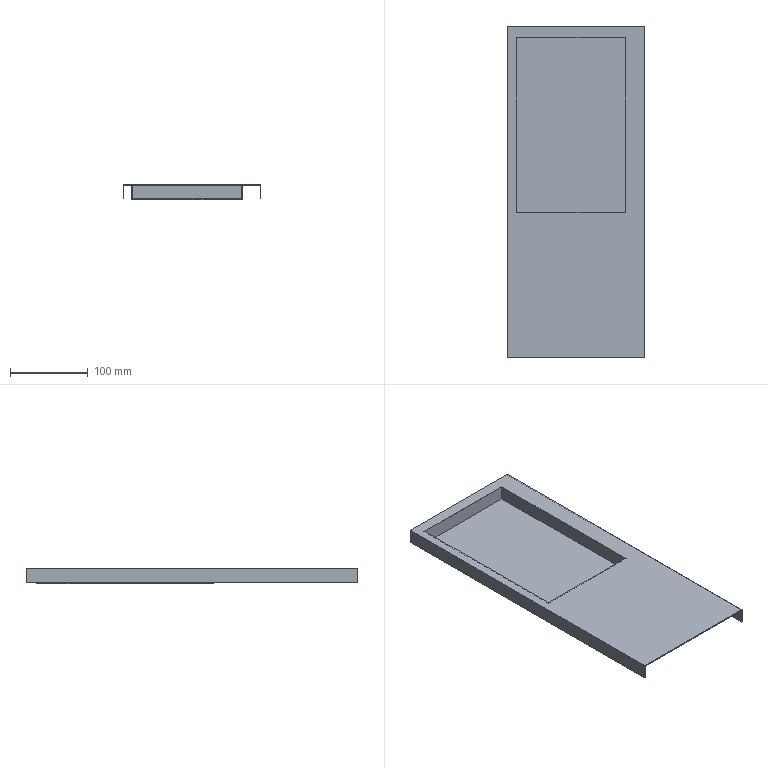Part | STEP file | Chassis front plate_RR | 1 solid | 20 faces | box 177 x 427 x 20 mm | volume 104897 mm3 | plane 20
STEP:
#1=CARTESIAN_POINT('',(0.,0.,0.));
#2=DIRECTION('',(0.,0.,1.));
#3=DIRECTION('',(1.,0.,0.));
#4=AXIS2_PLACEMENT_3D('',#1,#2,#3);
#5=CARTESIAN_POINT('',(-76.5,-26.5,0.));
#6=VERTEX_POINT('',#5);
#7=CARTESIAN_POINT('',(-76.5,198.5,0.));
#8=VERTEX_POINT('',#7);
#9=CARTESIAN_POINT('',(-76.5,-213.5,0.));
#10=DIRECTION('',(0.,1.,0.));
#11=VECTOR('',#10,1.);
#12=LINE('',#9,#11);
#13=CARTESIAN_POINT('',(-88.5,-213.5,0.));
#14=DIRECTION('',(0.,0.,1.));
#15=DIRECTION('',(1.,0.,0.));
#16=AXIS2_PLACEMENT_3D('',#13,#14,#15);
#17=PLANE('',#16);
#18=CARTESIAN_POINT('',(12.,0.));
#19=DIRECTION('',(0.,1.));
#20=VECTOR('',#19,1.);
#21=LINE('',#18,#20);
#22=(GEOMETRIC_REPRESENTATION_CONTEXT(2)PARAMETRIC_REPRESENTATION_CONTEXT()REPRESENTATION_CONTEXT('',''));
#23=DEFINITIONAL_REPRESENTATION('',(#21),#22);
#24=PCURVE('',#17,#23);
#25=CARTESIAN_POINT('',(-76.5,198.5,0.));
#26=DIRECTION('',(-1.,0.,0.));
#27=DIRECTION('',(0.,0.,1.));
#28=AXIS2_PLACEMENT_3D('',#25,#26,#27);
#29=PLANE('',#28);
#30=CARTESIAN_POINT('',(0.,-412.));
#31=DIRECTION('',(0.,1.));
#32=VECTOR('',#31,1.);
#33=LINE('',#30,#32);
#34=(GEOMETRIC_REPRESENTATION_CONTEXT(2)PARAMETRIC_REPRESENTATION_CONTEXT()REPRESENTATION_CONTEXT('',''));
#35=DEFINITIONAL_REPRESENTATION('',(#33),#34);
#36=PCURVE('',#29,#35);
#37=SURFACE_CURVE('',#12,(#24,#36),.PCURVE_S1.);
#38=EDGE_CURVE('',#6,#8,#37,.T.);
#39=ORIENTED_EDGE('',*,*,#38,.T.);
#40=CARTESIAN_POINT('',(63.5,198.5,0.));
#41=VERTEX_POINT('',#40);
#42=CARTESIAN_POINT('',(-88.5,198.5,0.));
#43=DIRECTION('',(1.,0.,0.));
#44=VECTOR('',#43,1.);
#45=LINE('',#42,#44);
#46=CARTESIAN_POINT('',(0.,412.));
#47=DIRECTION('',(1.,0.));
#48=VECTOR('',#47,1.);
#49=LINE('',#46,#48);
#50=(GEOMETRIC_REPRESENTATION_CONTEXT(2)PARAMETRIC_REPRESENTATION_CONTEXT()REPRESENTATION_CONTEXT('',''));
#51=DEFINITIONAL_REPRESENTATION('',(#49),#50);
#52=PCURVE('',#17,#51);
#53=CARTESIAN_POINT('',(63.5,198.5,0.));
#54=DIRECTION('',(0.,1.,0.));
#55=DIRECTION('',(0.,0.,1.));
#56=AXIS2_PLACEMENT_3D('',#53,#54,#55);
#57=PLANE('',#56);
#58=CARTESIAN_POINT('',(0.,-152.));
#59=DIRECTION('',(0.,1.));
#60=VECTOR('',#59,1.);
#61=LINE('',#58,#60);
#62=(GEOMETRIC_REPRESENTATION_CONTEXT(2)PARAMETRIC_REPRESENTATION_CONTEXT()REPRESENTATION_CONTEXT('',''));
#63=DEFINITIONAL_REPRESENTATION('',(#61),#62);
#64=PCURVE('',#57,#63);
#65=SURFACE_CURVE('',#45,(#52,#64),.PCURVE_S1.);
#66=EDGE_CURVE('',#8,#41,#65,.T.);
#67=ORIENTED_EDGE('',*,*,#66,.T.);
#68=CARTESIAN_POINT('',(63.5,-26.5,0.));
#69=VERTEX_POINT('',#68);
#70=CARTESIAN_POINT('',(63.5,-213.5,0.));
#71=DIRECTION('',(0.,-1.,0.));
#72=VECTOR('',#71,1.);
#73=LINE('',#70,#72);
#74=CARTESIAN_POINT('',(152.,0.));
#75=DIRECTION('',(0.,-1.));
#76=VECTOR('',#75,1.);
#77=LINE('',#74,#76);
#78=(GEOMETRIC_REPRESENTATION_CONTEXT(2)PARAMETRIC_REPRESENTATION_CONTEXT()REPRESENTATION_CONTEXT('',''));
#79=DEFINITIONAL_REPRESENTATION('',(#77),#78);
#80=PCURVE('',#17,#79);
#81=CARTESIAN_POINT('',(63.5,-26.5,0.));
#82=DIRECTION('',(1.,0.,0.));
#83=DIRECTION('',(0.,0.,-1.));
#84=AXIS2_PLACEMENT_3D('',#81,#82,#83);
#85=PLANE('',#84);
#86=CARTESIAN_POINT('',(0.,-187.));
#87=DIRECTION('',(0.,-1.));
#88=VECTOR('',#87,1.);
#89=LINE('',#86,#88);
#90=(GEOMETRIC_REPRESENTATION_CONTEXT(2)PARAMETRIC_REPRESENTATION_CONTEXT()REPRESENTATION_CONTEXT('',''));
#91=DEFINITIONAL_REPRESENTATION('',(#89),#90);
#92=PCURVE('',#85,#91);
#93=SURFACE_CURVE('',#73,(#80,#92),.PCURVE_S1.);
#94=EDGE_CURVE('',#41,#69,#93,.T.);
#95=ORIENTED_EDGE('',*,*,#94,.T.);
#96=CARTESIAN_POINT('',(-88.5,-26.5,0.));
#97=DIRECTION('',(-1.,0.,0.));
#98=VECTOR('',#97,1.);
#99=LINE('',#96,#98);
#100=CARTESIAN_POINT('',(0.,187.));
#101=DIRECTION('',(-1.,0.));
#102=VECTOR('',#101,1.);
#103=LINE('',#100,#102);
#104=(GEOMETRIC_REPRESENTATION_CONTEXT(2)PARAMETRIC_REPRESENTATION_CONTEXT()REPRESENTATION_CONTEXT('',''));
#105=DEFINITIONAL_REPRESENTATION('',(#103),#104);
#106=PCURVE('',#17,#105);
#107=CARTESIAN_POINT('',(-76.5,-26.5,0.));
#108=DIRECTION('',(0.,-1.,0.));
#109=DIRECTION('',(0.,0.,-1.));
#110=AXIS2_PLACEMENT_3D('',#107,#108,#109);
#111=PLANE('',#110);
#112=CARTESIAN_POINT('',(0.,-12.));
#113=DIRECTION('',(0.,-1.));
#114=VECTOR('',#113,1.);
#115=LINE('',#112,#114);
#116=(GEOMETRIC_REPRESENTATION_CONTEXT(2)PARAMETRIC_REPRESENTATION_CONTEXT()REPRESENTATION_CONTEXT('',''));
#117=DEFINITIONAL_REPRESENTATION('',(#115),#116);
#118=PCURVE('',#111,#117);
#119=SURFACE_CURVE('',#99,(#106,#118),.PCURVE_S1.);
#120=EDGE_CURVE('',#69,#6,#119,.T.);
#121=ORIENTED_EDGE('',*,*,#120,.T.);
#122=EDGE_LOOP('',(#39,#67,#95,#121));
#123=FACE_BOUND('',#122,.T.);
#124=CARTESIAN_POINT('',(-88.5,213.5,0.));
#125=VERTEX_POINT('',#124);
#126=CARTESIAN_POINT('',(-88.5,-213.5,0.));
#127=VERTEX_POINT('',#126);
#128=CARTESIAN_POINT('',(-88.5,-213.5,0.));
#129=DIRECTION('',(0.,-1.,0.));
#130=VECTOR('',#129,1.);
#131=LINE('',#128,#130);
#132=CARTESIAN_POINT('',(0.,0.));
#133=DIRECTION('',(0.,-1.));
#134=VECTOR('',#133,1.);
#135=LINE('',#132,#134);
#136=(GEOMETRIC_REPRESENTATION_CONTEXT(2)PARAMETRIC_REPRESENTATION_CONTEXT()REPRESENTATION_CONTEXT('',''));
#137=DEFINITIONAL_REPRESENTATION('',(#135),#136);
#138=PCURVE('',#17,#137);
#139=CARTESIAN_POINT('',(-88.5,-213.5,-19.));
#140=DIRECTION('',(-1.,0.,0.));
#141=DIRECTION('',(0.,0.,1.));
#142=AXIS2_PLACEMENT_3D('',#139,#140,#141);
#143=PLANE('',#142);
#144=CARTESIAN_POINT('',(19.,0.));
#145=DIRECTION('',(0.,-1.));
#146=VECTOR('',#145,1.);
#147=LINE('',#144,#146);
#148=(GEOMETRIC_REPRESENTATION_CONTEXT(2)PARAMETRIC_REPRESENTATION_CONTEXT()REPRESENTATION_CONTEXT('',''));
#149=DEFINITIONAL_REPRESENTATION('',(#147),#148);
#150=PCURVE('',#143,#149);
#151=SURFACE_CURVE('',#131,(#138,#150),.PCURVE_S1.);
#152=EDGE_CURVE('',#125,#127,#151,.T.);
#153=ORIENTED_EDGE('',*,*,#152,.T.);
#154=CARTESIAN_POINT('',(88.5,-213.5,0.));
#155=VERTEX_POINT('',#154);
#156=CARTESIAN_POINT('',(-88.5,-213.5,0.));
#157=DIRECTION('',(1.,0.,0.));
#158=VECTOR('',#157,1.);
#159=LINE('',#156,#158);
#160=CARTESIAN_POINT('',(0.,0.));
#161=DIRECTION('',(1.,0.));
#162=VECTOR('',#161,1.);
#163=LINE('',#160,#162);
#164=(GEOMETRIC_REPRESENTATION_CONTEXT(2)PARAMETRIC_REPRESENTATION_CONTEXT()REPRESENTATION_CONTEXT('',''));
#165=DEFINITIONAL_REPRESENTATION('',(#163),#164);
#166=PCURVE('',#17,#165);
#167=CARTESIAN_POINT('',(0.,-213.5,0.));
#168=DIRECTION('',(0.,1.,0.));
#169=DIRECTION('',(0.,0.,1.));
#170=AXIS2_PLACEMENT_3D('',#167,#168,#169);
#171=PLANE('',#170);
#172=CARTESIAN_POINT('',(0.,-88.5));
#173=DIRECTION('',(0.,1.));
#174=VECTOR('',#173,1.);
#175=LINE('',#172,#174);
#176=(GEOMETRIC_REPRESENTATION_CONTEXT(2)PARAMETRIC_REPRESENTATION_CONTEXT()REPRESENTATION_CONTEXT('',''));
#177=DEFINITIONAL_REPRESENTATION('',(#175),#176);
#178=PCURVE('',#171,#177);
#179=SURFACE_CURVE('',#159,(#166,#178),.PCURVE_S1.);
#180=EDGE_CURVE('',#127,#155,#179,.T.);
#181=ORIENTED_EDGE('',*,*,#180,.T.);
#182=CARTESIAN_POINT('',(88.5,213.5,0.));
#183=VERTEX_POINT('',#182);
#184=CARTESIAN_POINT('',(88.5,-213.5,0.));
#185=DIRECTION('',(0.,1.,0.));
#186=VECTOR('',#185,1.);
#187=LINE('',#184,#186);
#188=CARTESIAN_POINT('',(177.,0.));
#189=DIRECTION('',(0.,1.));
#190=VECTOR('',#189,1.);
#191=LINE('',#188,#190);
#192=(GEOMETRIC_REPRESENTATION_CONTEXT(2)PARAMETRIC_REPRESENTATION_CONTEXT()REPRESENTATION_CONTEXT('',''));
#193=DEFINITIONAL_REPRESENTATION('',(#191),#192);
#194=PCURVE('',#17,#193);
#195=CARTESIAN_POINT('',(88.5,-213.5,0.));
#196=DIRECTION('',(1.,0.,0.));
#197=DIRECTION('',(0.,0.,-1.));
#198=AXIS2_PLACEMENT_3D('',#195,#196,#197);
#199=PLANE('',#198);
#200=CARTESIAN_POINT('',(0.,0.));
#201=DIRECTION('',(0.,1.));
#202=VECTOR('',#201,1.);
#203=LINE('',#200,#202);
#204=(GEOMETRIC_REPRESENTATION_CONTEXT(2)PARAMETRIC_REPRESENTATION_CONTEXT()REPRESENTATION_CONTEXT('',''));
#205=DEFINITIONAL_REPRESENTATION('',(#203),#204);
#206=PCURVE('',#199,#205);
#207=SURFACE_CURVE('',#187,(#194,#206),.PCURVE_S1.);
#208=EDGE_CURVE('',#155,#183,#207,.T.);
#209=ORIENTED_EDGE('',*,*,#208,.T.);
#210=CARTESIAN_POINT('',(-88.5,213.5,0.));
#211=DIRECTION('',(-1.,0.,0.));
#212=VECTOR('',#211,1.);
#213=LINE('',#210,#212);
#214=CARTESIAN_POINT('',(0.,427.));
#215=DIRECTION('',(-1.,0.));
#216=VECTOR('',#215,1.);
#217=LINE('',#214,#216);
#218=(GEOMETRIC_REPRESENTATION_CONTEXT(2)PARAMETRIC_REPRESENTATION_CONTEXT()REPRESENTATION_CONTEXT('',''));
#219=DEFINITIONAL_REPRESENTATION('',(#217),#218);
#220=PCURVE('',#17,#219);
#221=CARTESIAN_POINT('',(0.,213.5,0.));
#222=DIRECTION('',(0.,1.,0.));
#223=DIRECTION('',(0.,0.,1.));
#224=AXIS2_PLACEMENT_3D('',#221,#222,#223);
#225=PLANE('',#224);
#226=CARTESIAN_POINT('',(0.,-88.5));
#227=DIRECTION('',(0.,-1.));
#228=VECTOR('',#227,1.);
#229=LINE('',#226,#228);
#230=(GEOMETRIC_REPRESENTATION_CONTEXT(2)PARAMETRIC_REPRESENTATION_CONTEXT()REPRESENTATION_CONTEXT('',''));
#231=DEFINITIONAL_REPRESENTATION('',(#229),#230);
#232=PCURVE('',#225,#231);
#233=SURFACE_CURVE('',#213,(#220,#232),.PCURVE_S1.);
#234=EDGE_CURVE('',#183,#125,#233,.T.);
#235=ORIENTED_EDGE('',*,*,#234,.T.);
#236=EDGE_LOOP('',(#153,#181,#209,#235));
#237=FACE_BOUND('',#236,.T.);
#238=ADVANCED_FACE('',(#123,#237),#17,.T.);
#239=ORIENTED_EDGE('',*,*,#66,.F.);
#240=CARTESIAN_POINT('',(-76.5,198.5,-19.));
#241=VERTEX_POINT('',#240);
#242=CARTESIAN_POINT('',(-76.5,198.5,0.));
#243=DIRECTION('',(0.,0.,1.));
#244=VECTOR('',#243,1.);
#245=LINE('',#242,#244);
#246=CARTESIAN_POINT('',(0.,-140.));
#247=DIRECTION('',(1.,0.));
#248=VECTOR('',#247,1.);
#249=LINE('',#246,#248);
#250=(GEOMETRIC_REPRESENTATION_CONTEXT(2)PARAMETRIC_REPRESENTATION_CONTEXT()REPRESENTATION_CONTEXT('',''));
#251=DEFINITIONAL_REPRESENTATION('',(#249),#250);
#252=PCURVE('',#57,#251);
#253=CARTESIAN_POINT('',(0.,0.));
#254=DIRECTION('',(1.,0.));
#255=VECTOR('',#254,1.);
#256=LINE('',#253,#255);
#257=(GEOMETRIC_REPRESENTATION_CONTEXT(2)PARAMETRIC_REPRESENTATION_CONTEXT()REPRESENTATION_CONTEXT('',''));
#258=DEFINITIONAL_REPRESENTATION('',(#256),#257);
#259=PCURVE('',#29,#258);
#260=SURFACE_CURVE('',#245,(#252,#259),.PCURVE_S1.);
#261=EDGE_CURVE('',#241,#8,#260,.T.);
#262=ORIENTED_EDGE('',*,*,#261,.F.);
#263=CARTESIAN_POINT('',(63.5,198.5,-19.));
#264=VERTEX_POINT('',#263);
#265=CARTESIAN_POINT('',(63.5,198.5,-19.));
#266=DIRECTION('',(-1.,0.,0.));
#267=VECTOR('',#266,1.);
#268=LINE('',#265,#267);
#269=CARTESIAN_POINT('',(-19.,0.));
#270=DIRECTION('',(0.,-1.));
#271=VECTOR('',#270,1.);
#272=LINE('',#269,#271);
#273=(GEOMETRIC_REPRESENTATION_CONTEXT(2)PARAMETRIC_REPRESENTATION_CONTEXT()REPRESENTATION_CONTEXT('',''));
#274=DEFINITIONAL_REPRESENTATION('',(#272),#273);
#275=PCURVE('',#57,#274);
#276=CARTESIAN_POINT('',(0.,-213.5,-19.));
#277=DIRECTION('',(0.,0.,-1.));
#278=DIRECTION('',(-1.,0.,0.));
#279=AXIS2_PLACEMENT_3D('',#276,#277,#278);
#280=PLANE('',#279);
#281=CARTESIAN_POINT('',(-63.5,412.));
#282=DIRECTION('',(1.,0.));
#283=VECTOR('',#282,1.);
#284=LINE('',#281,#283);
#285=(GEOMETRIC_REPRESENTATION_CONTEXT(2)PARAMETRIC_REPRESENTATION_CONTEXT()REPRESENTATION_CONTEXT('',''));
#286=DEFINITIONAL_REPRESENTATION('',(#284),#285);
#287=PCURVE('',#280,#286);
#288=SURFACE_CURVE('',#268,(#275,#287),.PCURVE_S1.);
#289=EDGE_CURVE('',#264,#241,#288,.T.);
#290=ORIENTED_EDGE('',*,*,#289,.F.);
#291=CARTESIAN_POINT('',(63.5,198.5,0.));
#292=DIRECTION('',(0.,0.,-1.));
#293=VECTOR('',#292,1.);
#294=LINE('',#291,#293);
#295=CARTESIAN_POINT('',(0.,0.));
#296=DIRECTION('',(-1.,0.));
#297=VECTOR('',#296,1.);
#298=LINE('',#295,#297);
#299=(GEOMETRIC_REPRESENTATION_CONTEXT(2)PARAMETRIC_REPRESENTATION_CONTEXT()REPRESENTATION_CONTEXT('',''));
#300=DEFINITIONAL_REPRESENTATION('',(#298),#299);
#301=PCURVE('',#57,#300);
#302=CARTESIAN_POINT('',(0.,225.));
#303=DIRECTION('',(1.,0.));
#304=VECTOR('',#303,1.);
#305=LINE('',#302,#304);
#306=(GEOMETRIC_REPRESENTATION_CONTEXT(2)PARAMETRIC_REPRESENTATION_CONTEXT()REPRESENTATION_CONTEXT('',''));
#307=DEFINITIONAL_REPRESENTATION('',(#305),#306);
#308=PCURVE('',#85,#307);
#309=SURFACE_CURVE('',#294,(#301,#308),.PCURVE_S1.);
#310=EDGE_CURVE('',#41,#264,#309,.T.);
#311=ORIENTED_EDGE('',*,*,#310,.F.);
#312=EDGE_LOOP('',(#239,#262,#290,#311));
#313=FACE_BOUND('',#312,.T.);
#314=ADVANCED_FACE('',(#313),#57,.F.);
#315=ORIENTED_EDGE('',*,*,#38,.F.);
#316=CARTESIAN_POINT('',(-76.5,-26.5,-19.));
#317=VERTEX_POINT('',#316);
#318=CARTESIAN_POINT('',(-76.5,-26.5,0.));
#319=DIRECTION('',(0.,0.,1.));
#320=VECTOR('',#319,1.);
#321=LINE('',#318,#320);
#322=CARTESIAN_POINT('',(0.,-225.));
#323=DIRECTION('',(1.,0.));
#324=VECTOR('',#323,1.);
#325=LINE('',#322,#324);
#326=(GEOMETRIC_REPRESENTATION_CONTEXT(2)PARAMETRIC_REPRESENTATION_CONTEXT()REPRESENTATION_CONTEXT('',''));
#327=DEFINITIONAL_REPRESENTATION('',(#325),#326);
#328=PCURVE('',#29,#327);
#329=CARTESIAN_POINT('',(0.,0.));
#330=DIRECTION('',(-1.,0.));
#331=VECTOR('',#330,1.);
#332=LINE('',#329,#331);
#333=(GEOMETRIC_REPRESENTATION_CONTEXT(2)PARAMETRIC_REPRESENTATION_CONTEXT()REPRESENTATION_CONTEXT('',''));
#334=DEFINITIONAL_REPRESENTATION('',(#332),#333);
#335=PCURVE('',#111,#334);
#336=SURFACE_CURVE('',#321,(#328,#335),.PCURVE_S1.);
#337=EDGE_CURVE('',#317,#6,#336,.T.);
#338=ORIENTED_EDGE('',*,*,#337,.F.);
#339=CARTESIAN_POINT('',(-76.5,198.5,-19.));
#340=DIRECTION('',(0.,-1.,0.));
#341=VECTOR('',#340,1.);
#342=LINE('',#339,#341);
#343=CARTESIAN_POINT('',(-19.,0.));
#344=DIRECTION('',(0.,-1.));
#345=VECTOR('',#344,1.);
#346=LINE('',#343,#345);
#347=(GEOMETRIC_REPRESENTATION_CONTEXT(2)PARAMETRIC_REPRESENTATION_CONTEXT()REPRESENTATION_CONTEXT('',''));
#348=DEFINITIONAL_REPRESENTATION('',(#346),#347);
#349=PCURVE('',#29,#348);
#350=CARTESIAN_POINT('',(76.5,412.));
#351=DIRECTION('',(0.,-1.));
#352=VECTOR('',#351,1.);
#353=LINE('',#350,#352);
#354=(GEOMETRIC_REPRESENTATION_CONTEXT(2)PARAMETRIC_REPRESENTATION_CONTEXT()REPRESENTATION_CONTEXT('',''));
#355=DEFINITIONAL_REPRESENTATION('',(#353),#354);
#356=PCURVE('',#280,#355);
#357=SURFACE_CURVE('',#342,(#349,#356),.PCURVE_S1.);
#358=EDGE_CURVE('',#241,#317,#357,.T.);
#359=ORIENTED_EDGE('',*,*,#358,.F.);
#360=ORIENTED_EDGE('',*,*,#261,.T.);
#361=EDGE_LOOP('',(#315,#338,#359,#360));
#362=FACE_BOUND('',#361,.T.);
#363=ADVANCED_FACE('',(#362),#29,.F.);
#364=ORIENTED_EDGE('',*,*,#120,.F.);
#365=CARTESIAN_POINT('',(63.5,-26.5,-19.));
#366=VERTEX_POINT('',#365);
#367=CARTESIAN_POINT('',(63.5,-26.5,0.));
#368=DIRECTION('',(0.,0.,1.));
#369=VECTOR('',#368,1.);
#370=LINE('',#367,#369);
#371=CARTESIAN_POINT('',(0.,140.));
#372=DIRECTION('',(-1.,0.));
#373=VECTOR('',#372,1.);
#374=LINE('',#371,#373);
#375=(GEOMETRIC_REPRESENTATION_CONTEXT(2)PARAMETRIC_REPRESENTATION_CONTEXT()REPRESENTATION_CONTEXT('',''));
#376=DEFINITIONAL_REPRESENTATION('',(#374),#375);
#377=PCURVE('',#111,#376);
#378=CARTESIAN_POINT('',(0.,0.));
#379=DIRECTION('',(-1.,0.));
#380=VECTOR('',#379,1.);
#381=LINE('',#378,#380);
#382=(GEOMETRIC_REPRESENTATION_CONTEXT(2)PARAMETRIC_REPRESENTATION_CONTEXT()REPRESENTATION_CONTEXT('',''));
#383=DEFINITIONAL_REPRESENTATION('',(#381),#382);
#384=PCURVE('',#85,#383);
#385=SURFACE_CURVE('',#370,(#377,#384),.PCURVE_S1.);
#386=EDGE_CURVE('',#366,#69,#385,.T.);
#387=ORIENTED_EDGE('',*,*,#386,.F.);
#388=CARTESIAN_POINT('',(-76.5,-26.5,-19.));
#389=DIRECTION('',(1.,0.,0.));
#390=VECTOR('',#389,1.);
#391=LINE('',#388,#390);
#392=CARTESIAN_POINT('',(19.,0.));
#393=DIRECTION('',(0.,1.));
#394=VECTOR('',#393,1.);
#395=LINE('',#392,#394);
#396=(GEOMETRIC_REPRESENTATION_CONTEXT(2)PARAMETRIC_REPRESENTATION_CONTEXT()REPRESENTATION_CONTEXT('',''));
#397=DEFINITIONAL_REPRESENTATION('',(#395),#396);
#398=PCURVE('',#111,#397);
#399=CARTESIAN_POINT('',(76.5,187.));
#400=DIRECTION('',(-1.,0.));
#401=VECTOR('',#400,1.);
#402=LINE('',#399,#401);
#403=(GEOMETRIC_REPRESENTATION_CONTEXT(2)PARAMETRIC_REPRESENTATION_CONTEXT()REPRESENTATION_CONTEXT('',''));
#404=DEFINITIONAL_REPRESENTATION('',(#402),#403);
#405=PCURVE('',#280,#404);
#406=SURFACE_CURVE('',#391,(#398,#405),.PCURVE_S1.);
#407=EDGE_CURVE('',#317,#366,#406,.T.);
#408=ORIENTED_EDGE('',*,*,#407,.F.);
#409=ORIENTED_EDGE('',*,*,#337,.T.);
#410=EDGE_LOOP('',(#364,#387,#408,#409));
#411=FACE_BOUND('',#410,.T.);
#412=ADVANCED_FACE('',(#411),#111,.F.);
#413=ORIENTED_EDGE('',*,*,#94,.F.);
#414=ORIENTED_EDGE('',*,*,#310,.T.);
#415=CARTESIAN_POINT('',(63.5,-26.5,-19.));
#416=DIRECTION('',(0.,1.,0.));
#417=VECTOR('',#416,1.);
#418=LINE('',#415,#417);
#419=CARTESIAN_POINT('',(19.,0.));
#420=DIRECTION('',(0.,1.));
#421=VECTOR('',#420,1.);
#422=LINE('',#419,#421);
#423=(GEOMETRIC_REPRESENTATION_CONTEXT(2)PARAMETRIC_REPRESENTATION_CONTEXT()REPRESENTATION_CONTEXT('',''));
#424=DEFINITIONAL_REPRESENTATION('',(#422),#423);
#425=PCURVE('',#85,#424);
#426=CARTESIAN_POINT('',(-63.5,187.));
#427=DIRECTION('',(0.,1.));
#428=VECTOR('',#427,1.);
#429=LINE('',#426,#428);
#430=(GEOMETRIC_REPRESENTATION_CONTEXT(2)PARAMETRIC_REPRESENTATION_CONTEXT()REPRESENTATION_CONTEXT('',''));
#431=DEFINITIONAL_REPRESENTATION('',(#429),#430);
#432=PCURVE('',#280,#431);
#433=SURFACE_CURVE('',#418,(#425,#432),.PCURVE_S1.);
#434=EDGE_CURVE('',#366,#264,#433,.T.);
#435=ORIENTED_EDGE('',*,*,#434,.F.);
#436=ORIENTED_EDGE('',*,*,#386,.T.);
#437=EDGE_LOOP('',(#413,#414,#435,#436));
#438=FACE_BOUND('',#437,.T.);
#439=ADVANCED_FACE('',(#438),#85,.F.);
#440=CARTESIAN_POINT('',(-87.5,-213.5,-1.));
#441=VERTEX_POINT('',#440);
#442=CARTESIAN_POINT('',(-87.5,-213.5,-19.));
#443=VERTEX_POINT('',#442);
#444=CARTESIAN_POINT('',(-87.5,-213.5,0.));
#445=DIRECTION('',(0.,0.,-1.));
#446=VECTOR('',#445,1.);
#447=LINE('',#444,#446);
#448=CARTESIAN_POINT('',(0.,-87.5));
#449=DIRECTION('',(-1.,0.));
#450=VECTOR('',#449,1.);
#451=LINE('',#448,#450);
#452=(GEOMETRIC_REPRESENTATION_CONTEXT(2)PARAMETRIC_REPRESENTATION_CONTEXT()REPRESENTATION_CONTEXT('',''));
#453=DEFINITIONAL_REPRESENTATION('',(#451),#452);
#454=PCURVE('',#171,#453);
#455=CARTESIAN_POINT('',(-87.5,-213.5,-1.));
#456=DIRECTION('',(1.,0.,0.));
#457=DIRECTION('',(0.,0.,-1.));
#458=AXIS2_PLACEMENT_3D('',#455,#456,#457);
#459=PLANE('',#458);
#460=CARTESIAN_POINT('',(-1.,0.));
#461=DIRECTION('',(1.,0.));
#462=VECTOR('',#461,1.);
#463=LINE('',#460,#462);
#464=(GEOMETRIC_REPRESENTATION_CONTEXT(2)PARAMETRIC_REPRESENTATION_CONTEXT()REPRESENTATION_CONTEXT('',''));
#465=DEFINITIONAL_REPRESENTATION('',(#463),#464);
#466=PCURVE('',#459,#465);
#467=SURFACE_CURVE('',#447,(#454,#466),.PCURVE_S1.);
#468=EDGE_CURVE('',#441,#443,#467,.T.);
#469=ORIENTED_EDGE('',*,*,#468,.F.);
#470=CARTESIAN_POINT('',(87.5,-213.5,-1.));
#471=VERTEX_POINT('',#470);
#472=CARTESIAN_POINT('',(0.,-213.5,-1.));
#473=DIRECTION('',(-1.,0.,0.));
#474=VECTOR('',#473,1.);
#475=LINE('',#472,#474);
#476=CARTESIAN_POINT('',(-1.,0.));
#477=DIRECTION('',(0.,-1.));
#478=VECTOR('',#477,1.);
#479=LINE('',#476,#478);
#480=(GEOMETRIC_REPRESENTATION_CONTEXT(2)PARAMETRIC_REPRESENTATION_CONTEXT()REPRESENTATION_CONTEXT('',''));
#481=DEFINITIONAL_REPRESENTATION('',(#479),#480);
#482=PCURVE('',#171,#481);
#483=CARTESIAN_POINT('',(87.5,-213.5,-1.));
#484=DIRECTION('',(0.,0.,-1.));
#485=DIRECTION('',(-1.,0.,0.));
#486=AXIS2_PLACEMENT_3D('',#483,#484,#485);
#487=PLANE('',#486);
#488=CARTESIAN_POINT('',(87.5,0.));
#489=DIRECTION('',(1.,0.));
#490=VECTOR('',#489,1.);
#491=LINE('',#488,#490);
#492=(GEOMETRIC_REPRESENTATION_CONTEXT(2)PARAMETRIC_REPRESENTATION_CONTEXT()REPRESENTATION_CONTEXT('',''));
#493=DEFINITIONAL_REPRESENTATION('',(#491),#492);
#494=PCURVE('',#487,#493);
#495=SURFACE_CURVE('',#475,(#482,#494),.PCURVE_S1.);
#496=EDGE_CURVE('',#471,#441,#495,.T.);
#497=ORIENTED_EDGE('',*,*,#496,.F.);
#498=CARTESIAN_POINT('',(87.5,-213.5,-19.));
#499=VERTEX_POINT('',#498);
#500=CARTESIAN_POINT('',(87.5,-213.5,0.));
#501=DIRECTION('',(0.,0.,1.));
#502=VECTOR('',#501,1.);
#503=LINE('',#500,#502);
#504=CARTESIAN_POINT('',(0.,87.5));
#505=DIRECTION('',(1.,0.));
#506=VECTOR('',#505,1.);
#507=LINE('',#504,#506);
#508=(GEOMETRIC_REPRESENTATION_CONTEXT(2)PARAMETRIC_REPRESENTATION_CONTEXT()REPRESENTATION_CONTEXT('',''));
#509=DEFINITIONAL_REPRESENTATION('',(#507),#508);
#510=PCURVE('',#171,#509);
#511=CARTESIAN_POINT('',(87.5,-213.5,-19.));
#512=DIRECTION('',(-1.,0.,0.));
#513=DIRECTION('',(0.,0.,1.));
#514=AXIS2_PLACEMENT_3D('',#511,#512,#513);
#515=PLANE('',#514);
#516=CARTESIAN_POINT('',(19.,0.));
#517=DIRECTION('',(1.,0.));
#518=VECTOR('',#517,1.);
#519=LINE('',#516,#518);
#520=(GEOMETRIC_REPRESENTATION_CONTEXT(2)PARAMETRIC_REPRESENTATION_CONTEXT()REPRESENTATION_CONTEXT('',''));
#521=DEFINITIONAL_REPRESENTATION('',(#519),#520);
#522=PCURVE('',#515,#521);
#523=SURFACE_CURVE('',#503,(#510,#522),.PCURVE_S1.);
#524=EDGE_CURVE('',#499,#471,#523,.T.);
#525=ORIENTED_EDGE('',*,*,#524,.F.);
#526=CARTESIAN_POINT('',(88.5,-213.5,-19.));
#527=VERTEX_POINT('',#526);
#528=CARTESIAN_POINT('',(88.5,-213.5,-19.));
#529=DIRECTION('',(-1.,0.,0.));
#530=VECTOR('',#529,1.);
#531=LINE('',#528,#530);
#532=CARTESIAN_POINT('',(-19.,88.5));
#533=DIRECTION('',(0.,-1.));
#534=VECTOR('',#533,1.);
#535=LINE('',#532,#534);
#536=(GEOMETRIC_REPRESENTATION_CONTEXT(2)PARAMETRIC_REPRESENTATION_CONTEXT()REPRESENTATION_CONTEXT('',''));
#537=DEFINITIONAL_REPRESENTATION('',(#535),#536);
#538=PCURVE('',#171,#537);
#539=CARTESIAN_POINT('',(88.5,-213.5,-19.));
#540=DIRECTION('',(0.,0.,-1.));
#541=DIRECTION('',(-1.,0.,0.));
#542=AXIS2_PLACEMENT_3D('',#539,#540,#541);
#543=PLANE('',#542);
#544=CARTESIAN_POINT('',(0.,0.));
#545=DIRECTION('',(1.,0.));
#546=VECTOR('',#545,1.);
#547=LINE('',#544,#546);
#548=(GEOMETRIC_REPRESENTATION_CONTEXT(2)PARAMETRIC_REPRESENTATION_CONTEXT()REPRESENTATION_CONTEXT('',''));
#549=DEFINITIONAL_REPRESENTATION('',(#547),#548);
#550=PCURVE('',#543,#549);
#551=SURFACE_CURVE('',#531,(#538,#550),.PCURVE_S1.);
#552=EDGE_CURVE('',#527,#499,#551,.T.);
#553=ORIENTED_EDGE('',*,*,#552,.F.);
#554=CARTESIAN_POINT('',(88.5,-213.5,0.));
#555=DIRECTION('',(0.,0.,-1.));
#556=VECTOR('',#555,1.);
#557=LINE('',#554,#556);
#558=CARTESIAN_POINT('',(0.,88.5));
#559=DIRECTION('',(-1.,0.));
#560=VECTOR('',#559,1.);
#561=LINE('',#558,#560);
#562=(GEOMETRIC_REPRESENTATION_CONTEXT(2)PARAMETRIC_REPRESENTATION_CONTEXT()REPRESENTATION_CONTEXT('',''));
#563=DEFINITIONAL_REPRESENTATION('',(#561),#562);
#564=PCURVE('',#171,#563);
#565=CARTESIAN_POINT('',(0.,0.));
#566=DIRECTION('',(1.,0.));
#567=VECTOR('',#566,1.);
#568=LINE('',#565,#567);
#569=(GEOMETRIC_REPRESENTATION_CONTEXT(2)PARAMETRIC_REPRESENTATION_CONTEXT()REPRESENTATION_CONTEXT('',''));
#570=DEFINITIONAL_REPRESENTATION('',(#568),#569);
#571=PCURVE('',#199,#570);
#572=SURFACE_CURVE('',#557,(#564,#571),.PCURVE_S1.);
#573=EDGE_CURVE('',#155,#527,#572,.T.);
#574=ORIENTED_EDGE('',*,*,#573,.F.);
#575=ORIENTED_EDGE('',*,*,#180,.F.);
#576=CARTESIAN_POINT('',(-88.5,-213.5,-19.));
#577=VERTEX_POINT('',#576);
#578=CARTESIAN_POINT('',(-88.5,-213.5,0.));
#579=DIRECTION('',(0.,0.,1.));
#580=VECTOR('',#579,1.);
#581=LINE('',#578,#580);
#582=CARTESIAN_POINT('',(0.,-88.5));
#583=DIRECTION('',(1.,0.));
#584=VECTOR('',#583,1.);
#585=LINE('',#582,#584);
#586=(GEOMETRIC_REPRESENTATION_CONTEXT(2)PARAMETRIC_REPRESENTATION_CONTEXT()REPRESENTATION_CONTEXT('',''));
#587=DEFINITIONAL_REPRESENTATION('',(#585),#586);
#588=PCURVE('',#171,#587);
#589=CARTESIAN_POINT('',(19.,0.));
#590=DIRECTION('',(1.,0.));
#591=VECTOR('',#590,1.);
#592=LINE('',#589,#591);
#593=(GEOMETRIC_REPRESENTATION_CONTEXT(2)PARAMETRIC_REPRESENTATION_CONTEXT()REPRESENTATION_CONTEXT('',''));
#594=DEFINITIONAL_REPRESENTATION('',(#592),#593);
#595=PCURVE('',#143,#594);
#596=SURFACE_CURVE('',#581,(#588,#595),.PCURVE_S1.);
#597=EDGE_CURVE('',#577,#127,#596,.T.);
#598=ORIENTED_EDGE('',*,*,#597,.F.);
#599=CARTESIAN_POINT('',(-87.5,-213.5,-19.));
#600=DIRECTION('',(-1.,0.,0.));
#601=VECTOR('',#600,1.);
#602=LINE('',#599,#601);
#603=CARTESIAN_POINT('',(-19.,-87.5));
#604=DIRECTION('',(0.,-1.));
#605=VECTOR('',#604,1.);
#606=LINE('',#603,#605);
#607=(GEOMETRIC_REPRESENTATION_CONTEXT(2)PARAMETRIC_REPRESENTATION_CONTEXT()REPRESENTATION_CONTEXT('',''));
#608=DEFINITIONAL_REPRESENTATION('',(#606),#607);
#609=PCURVE('',#171,#608);
#610=CARTESIAN_POINT('',(-87.5,-213.5,-19.));
#611=DIRECTION('',(0.,0.,-1.));
#612=DIRECTION('',(-1.,0.,0.));
#613=AXIS2_PLACEMENT_3D('',#610,#611,#612);
#614=PLANE('',#613);
#615=CARTESIAN_POINT('',(0.,0.));
#616=DIRECTION('',(1.,0.));
#617=VECTOR('',#616,1.);
#618=LINE('',#615,#617);
#619=(GEOMETRIC_REPRESENTATION_CONTEXT(2)PARAMETRIC_REPRESENTATION_CONTEXT()REPRESENTATION_CONTEXT('',''));
#620=DEFINITIONAL_REPRESENTATION('',(#618),#619);
#621=PCURVE('',#614,#620);
#622=SURFACE_CURVE('',#602,(#609,#621),.PCURVE_S1.);
#623=EDGE_CURVE('',#443,#577,#622,.T.);
#624=ORIENTED_EDGE('',*,*,#623,.F.);
#625=EDGE_LOOP('',(#469,#497,#525,#553,#574,#575,#598,#624));
#626=FACE_BOUND('',#625,.T.);
#627=ADVANCED_FACE('',(#626),#171,.F.);
#628=CARTESIAN_POINT('',(-88.5,213.5,-19.));
#629=VERTEX_POINT('',#628);
#630=CARTESIAN_POINT('',(-88.5,-213.5,-19.));
#631=DIRECTION('',(0.,-1.,0.));
#632=VECTOR('',#631,1.);
#633=LINE('',#630,#632);
#634=CARTESIAN_POINT('',(0.,0.));
#635=DIRECTION('',(0.,-1.));
#636=VECTOR('',#635,1.);
#637=LINE('',#634,#636);
#638=(GEOMETRIC_REPRESENTATION_CONTEXT(2)PARAMETRIC_REPRESENTATION_CONTEXT()REPRESENTATION_CONTEXT('',''));
#639=DEFINITIONAL_REPRESENTATION('',(#637),#638);
#640=PCURVE('',#143,#639);
#641=CARTESIAN_POINT('',(1.,0.));
#642=DIRECTION('',(0.,-1.));
#643=VECTOR('',#642,1.);
#644=LINE('',#641,#643);
#645=(GEOMETRIC_REPRESENTATION_CONTEXT(2)PARAMETRIC_REPRESENTATION_CONTEXT()REPRESENTATION_CONTEXT('',''));
#646=DEFINITIONAL_REPRESENTATION('',(#644),#645);
#647=PCURVE('',#614,#646);
#648=SURFACE_CURVE('',#633,(#640,#647),.PCURVE_S1.);
#649=EDGE_CURVE('',#629,#577,#648,.T.);
#650=ORIENTED_EDGE('',*,*,#649,.T.);
#651=ORIENTED_EDGE('',*,*,#597,.T.);
#652=ORIENTED_EDGE('',*,*,#152,.F.);
#653=CARTESIAN_POINT('',(-88.5,213.5,-19.));
#654=DIRECTION('',(0.,0.,-1.));
#655=VECTOR('',#654,1.);
#656=LINE('',#653,#655);
#657=CARTESIAN_POINT('',(0.,427.));
#658=DIRECTION('',(-1.,0.));
#659=VECTOR('',#658,1.);
#660=LINE('',#657,#659);
#661=(GEOMETRIC_REPRESENTATION_CONTEXT(2)PARAMETRIC_REPRESENTATION_CONTEXT()REPRESENTATION_CONTEXT('',''));
#662=DEFINITIONAL_REPRESENTATION('',(#660),#661);
#663=PCURVE('',#143,#662);
#664=CARTESIAN_POINT('',(-19.,-88.5));
#665=DIRECTION('',(-1.,0.));
#666=VECTOR('',#665,1.);
#667=LINE('',#664,#666);
#668=(GEOMETRIC_REPRESENTATION_CONTEXT(2)PARAMETRIC_REPRESENTATION_CONTEXT()REPRESENTATION_CONTEXT('',''));
#669=DEFINITIONAL_REPRESENTATION('',(#667),#668);
#670=PCURVE('',#225,#669);
#671=SURFACE_CURVE('',#656,(#663,#670),.PCURVE_S1.);
#672=EDGE_CURVE('',#125,#629,#671,.T.);
#673=ORIENTED_EDGE('',*,*,#672,.T.);
#674=EDGE_LOOP('',(#650,#651,#652,#673));
#675=FACE_BOUND('',#674,.T.);
#676=ADVANCED_FACE('',(#675),#143,.T.);
#677=CARTESIAN_POINT('',(-87.5,213.5,-19.));
#678=VERTEX_POINT('',#677);
#679=CARTESIAN_POINT('',(0.,213.5,-19.));
#680=DIRECTION('',(-1.,0.,0.));
#681=VECTOR('',#680,1.);
#682=LINE('',#679,#681);
#683=CARTESIAN_POINT('',(-19.,0.));
#684=DIRECTION('',(0.,-1.));
#685=VECTOR('',#684,1.);
#686=LINE('',#683,#685);
#687=(GEOMETRIC_REPRESENTATION_CONTEXT(2)PARAMETRIC_REPRESENTATION_CONTEXT()REPRESENTATION_CONTEXT('',''));
#688=DEFINITIONAL_REPRESENTATION('',(#686),#687);
#689=PCURVE('',#225,#688);
#690=CARTESIAN_POINT('',(-87.5,427.));
#691=DIRECTION('',(1.,0.));
#692=VECTOR('',#691,1.);
#693=LINE('',#690,#692);
#694=(GEOMETRIC_REPRESENTATION_CONTEXT(2)PARAMETRIC_REPRESENTATION_CONTEXT()REPRESENTATION_CONTEXT('',''));
#695=DEFINITIONAL_REPRESENTATION('',(#693),#694);
#696=PCURVE('',#614,#695);
#697=SURFACE_CURVE('',#682,(#689,#696),.PCURVE_S1.);
#698=EDGE_CURVE('',#678,#629,#697,.T.);
#699=ORIENTED_EDGE('',*,*,#698,.T.);
#700=ORIENTED_EDGE('',*,*,#672,.F.);
#701=ORIENTED_EDGE('',*,*,#234,.F.);
#702=CARTESIAN_POINT('',(88.5,213.5,-19.));
#703=VERTEX_POINT('',#702);
#704=CARTESIAN_POINT('',(88.5,213.5,0.));
#705=DIRECTION('',(0.,0.,-1.));
#706=VECTOR('',#705,1.);
#707=LINE('',#704,#706);
#708=CARTESIAN_POINT('',(0.,88.5));
#709=DIRECTION('',(-1.,0.));
#710=VECTOR('',#709,1.);
#711=LINE('',#708,#710);
#712=(GEOMETRIC_REPRESENTATION_CONTEXT(2)PARAMETRIC_REPRESENTATION_CONTEXT()REPRESENTATION_CONTEXT('',''));
#713=DEFINITIONAL_REPRESENTATION('',(#711),#712);
#714=PCURVE('',#225,#713);
#715=CARTESIAN_POINT('',(0.,427.));
#716=DIRECTION('',(1.,0.));
#717=VECTOR('',#716,1.);
#718=LINE('',#715,#717);
#719=(GEOMETRIC_REPRESENTATION_CONTEXT(2)PARAMETRIC_REPRESENTATION_CONTEXT()REPRESENTATION_CONTEXT('',''));
#720=DEFINITIONAL_REPRESENTATION('',(#718),#719);
#721=PCURVE('',#199,#720);
#722=SURFACE_CURVE('',#707,(#714,#721),.PCURVE_S1.);
#723=EDGE_CURVE('',#183,#703,#722,.T.);
#724=ORIENTED_EDGE('',*,*,#723,.T.);
#725=CARTESIAN_POINT('',(87.5,213.5,-19.));
#726=VERTEX_POINT('',#725);
#727=CARTESIAN_POINT('',(88.5,213.5,-19.));
#728=DIRECTION('',(1.,0.,0.));
#729=VECTOR('',#728,1.);
#730=LINE('',#727,#729);
#731=CARTESIAN_POINT('',(-19.,88.5));
#732=DIRECTION('',(0.,1.));
#733=VECTOR('',#732,1.);
#734=LINE('',#731,#733);
#735=(GEOMETRIC_REPRESENTATION_CONTEXT(2)PARAMETRIC_REPRESENTATION_CONTEXT()REPRESENTATION_CONTEXT('',''));
#736=DEFINITIONAL_REPRESENTATION('',(#734),#735);
#737=PCURVE('',#225,#736);
#738=CARTESIAN_POINT('',(0.,427.));
#739=DIRECTION('',(-1.,0.));
#740=VECTOR('',#739,1.);
#741=LINE('',#738,#740);
#742=(GEOMETRIC_REPRESENTATION_CONTEXT(2)PARAMETRIC_REPRESENTATION_CONTEXT()REPRESENTATION_CONTEXT('',''));
#743=DEFINITIONAL_REPRESENTATION('',(#741),#742);
#744=PCURVE('',#543,#743);
#745=SURFACE_CURVE('',#730,(#737,#744),.PCURVE_S1.);
#746=EDGE_CURVE('',#726,#703,#745,.T.);
#747=ORIENTED_EDGE('',*,*,#746,.F.);
#748=CARTESIAN_POINT('',(87.5,213.5,-1.));
#749=VERTEX_POINT('',#748);
#750=CARTESIAN_POINT('',(87.5,213.5,0.));
#751=DIRECTION('',(0.,0.,1.));
#752=VECTOR('',#751,1.);
#753=LINE('',#750,#752);
#754=CARTESIAN_POINT('',(0.,87.5));
#755=DIRECTION('',(1.,0.));
#756=VECTOR('',#755,1.);
#757=LINE('',#754,#756);
#758=(GEOMETRIC_REPRESENTATION_CONTEXT(2)PARAMETRIC_REPRESENTATION_CONTEXT()REPRESENTATION_CONTEXT('',''));
#759=DEFINITIONAL_REPRESENTATION('',(#757),#758);
#760=PCURVE('',#225,#759);
#761=CARTESIAN_POINT('',(19.,427.));
#762=DIRECTION('',(1.,0.));
#763=VECTOR('',#762,1.);
#764=LINE('',#761,#763);
#765=(GEOMETRIC_REPRESENTATION_CONTEXT(2)PARAMETRIC_REPRESENTATION_CONTEXT()REPRESENTATION_CONTEXT('',''));
#766=DEFINITIONAL_REPRESENTATION('',(#764),#765);
#767=PCURVE('',#515,#766);
#768=SURFACE_CURVE('',#753,(#760,#767),.PCURVE_S1.);
#769=EDGE_CURVE('',#726,#749,#768,.T.);
#770=ORIENTED_EDGE('',*,*,#769,.T.);
#771=CARTESIAN_POINT('',(-87.5,213.5,-1.));
#772=VERTEX_POINT('',#771);
#773=CARTESIAN_POINT('',(0.,213.5,-1.));
#774=DIRECTION('',(-1.,0.,0.));
#775=VECTOR('',#774,1.);
#776=LINE('',#773,#775);
#777=CARTESIAN_POINT('',(-1.,0.));
#778=DIRECTION('',(0.,-1.));
#779=VECTOR('',#778,1.);
#780=LINE('',#777,#779);
#781=(GEOMETRIC_REPRESENTATION_CONTEXT(2)PARAMETRIC_REPRESENTATION_CONTEXT()REPRESENTATION_CONTEXT('',''));
#782=DEFINITIONAL_REPRESENTATION('',(#780),#781);
#783=PCURVE('',#225,#782);
#784=CARTESIAN_POINT('',(87.5,427.));
#785=DIRECTION('',(1.,0.));
#786=VECTOR('',#785,1.);
#787=LINE('',#784,#786);
#788=(GEOMETRIC_REPRESENTATION_CONTEXT(2)PARAMETRIC_REPRESENTATION_CONTEXT()REPRESENTATION_CONTEXT('',''));
#789=DEFINITIONAL_REPRESENTATION('',(#787),#788);
#790=PCURVE('',#487,#789);
#791=SURFACE_CURVE('',#776,(#783,#790),.PCURVE_S1.);
#792=EDGE_CURVE('',#749,#772,#791,.T.);
#793=ORIENTED_EDGE('',*,*,#792,.T.);
#794=CARTESIAN_POINT('',(-87.5,213.5,0.));
#795=DIRECTION('',(0.,0.,-1.));
#796=VECTOR('',#795,1.);
#797=LINE('',#794,#796);
#798=CARTESIAN_POINT('',(0.,-87.5));
#799=DIRECTION('',(-1.,0.));
#800=VECTOR('',#799,1.);
#801=LINE('',#798,#800);
#802=(GEOMETRIC_REPRESENTATION_CONTEXT(2)PARAMETRIC_REPRESENTATION_CONTEXT()REPRESENTATION_CONTEXT('',''));
#803=DEFINITIONAL_REPRESENTATION('',(#801),#802);
#804=PCURVE('',#225,#803);
#805=CARTESIAN_POINT('',(-1.,427.));
#806=DIRECTION('',(1.,0.));
#807=VECTOR('',#806,1.);
#808=LINE('',#805,#807);
#809=(GEOMETRIC_REPRESENTATION_CONTEXT(2)PARAMETRIC_REPRESENTATION_CONTEXT()REPRESENTATION_CONTEXT('',''));
#810=DEFINITIONAL_REPRESENTATION('',(#808),#809);
#811=PCURVE('',#459,#810);
#812=SURFACE_CURVE('',#797,(#804,#811),.PCURVE_S1.);
#813=EDGE_CURVE('',#772,#678,#812,.T.);
#814=ORIENTED_EDGE('',*,*,#813,.T.);
#815=EDGE_LOOP('',(#699,#700,#701,#724,#747,#770,#793,#814));
#816=FACE_BOUND('',#815,.T.);
#817=ADVANCED_FACE('',(#816),#225,.T.);
#818=ORIENTED_EDGE('',*,*,#208,.F.);
#819=ORIENTED_EDGE('',*,*,#573,.T.);
#820=CARTESIAN_POINT('',(88.5,-213.5,-19.));
#821=DIRECTION('',(0.,1.,0.));
#822=VECTOR('',#821,1.);
#823=LINE('',#820,#822);
#824=CARTESIAN_POINT('',(19.,0.));
#825=DIRECTION('',(0.,1.));
#826=VECTOR('',#825,1.);
#827=LINE('',#824,#826);
#828=(GEOMETRIC_REPRESENTATION_CONTEXT(2)PARAMETRIC_REPRESENTATION_CONTEXT()REPRESENTATION_CONTEXT('',''));
#829=DEFINITIONAL_REPRESENTATION('',(#827),#828);
#830=PCURVE('',#199,#829);
#831=CARTESIAN_POINT('',(0.,0.));
#832=DIRECTION('',(0.,1.));
#833=VECTOR('',#832,1.);
#834=LINE('',#831,#833);
#835=(GEOMETRIC_REPRESENTATION_CONTEXT(2)PARAMETRIC_REPRESENTATION_CONTEXT()REPRESENTATION_CONTEXT('',''));
#836=DEFINITIONAL_REPRESENTATION('',(#834),#835);
#837=PCURVE('',#543,#836);
#838=SURFACE_CURVE('',#823,(#830,#837),.PCURVE_S1.);
#839=EDGE_CURVE('',#527,#703,#838,.T.);
#840=ORIENTED_EDGE('',*,*,#839,.T.);
#841=ORIENTED_EDGE('',*,*,#723,.F.);
#842=EDGE_LOOP('',(#818,#819,#840,#841));
#843=FACE_BOUND('',#842,.T.);
#844=ADVANCED_FACE('',(#843),#199,.T.);
#845=ORIENTED_EDGE('',*,*,#407,.T.);
#846=ORIENTED_EDGE('',*,*,#434,.T.);
#847=ORIENTED_EDGE('',*,*,#289,.T.);
#848=ORIENTED_EDGE('',*,*,#358,.T.);
#849=EDGE_LOOP('',(#845,#846,#847,#848));
#850=FACE_BOUND('',#849,.T.);
#851=ADVANCED_FACE('',(#850),#280,.F.);
#852=CARTESIAN_POINT('',(-87.5,-213.5,-1.));
#853=DIRECTION('',(0.,-1.,0.));
#854=VECTOR('',#853,1.);
#855=LINE('',#852,#854);
#856=CARTESIAN_POINT('',(0.,0.));
#857=DIRECTION('',(0.,-1.));
#858=VECTOR('',#857,1.);
#859=LINE('',#856,#858);
#860=(GEOMETRIC_REPRESENTATION_CONTEXT(2)PARAMETRIC_REPRESENTATION_CONTEXT()REPRESENTATION_CONTEXT('',''));
#861=DEFINITIONAL_REPRESENTATION('',(#859),#860);
#862=PCURVE('',#459,#861);
#863=CARTESIAN_POINT('',(175.,0.));
#864=DIRECTION('',(0.,-1.));
#865=VECTOR('',#864,1.);
#866=LINE('',#863,#865);
#867=(GEOMETRIC_REPRESENTATION_CONTEXT(2)PARAMETRIC_REPRESENTATION_CONTEXT()REPRESENTATION_CONTEXT('',''));
#868=DEFINITIONAL_REPRESENTATION('',(#866),#867);
#869=PCURVE('',#487,#868);
#870=SURFACE_CURVE('',#855,(#862,#869),.PCURVE_S1.);
#871=EDGE_CURVE('',#772,#441,#870,.T.);
#872=ORIENTED_EDGE('',*,*,#871,.T.);
#873=ORIENTED_EDGE('',*,*,#468,.T.);
#874=CARTESIAN_POINT('',(-87.5,-213.5,-19.));
#875=DIRECTION('',(0.,1.,0.));
#876=VECTOR('',#875,1.);
#877=LINE('',#874,#876);
#878=CARTESIAN_POINT('',(18.,0.));
#879=DIRECTION('',(0.,1.));
#880=VECTOR('',#879,1.);
#881=LINE('',#878,#880);
#882=(GEOMETRIC_REPRESENTATION_CONTEXT(2)PARAMETRIC_REPRESENTATION_CONTEXT()REPRESENTATION_CONTEXT('',''));
#883=DEFINITIONAL_REPRESENTATION('',(#881),#882);
#884=PCURVE('',#459,#883);
#885=CARTESIAN_POINT('',(0.,0.));
#886=DIRECTION('',(0.,1.));
#887=VECTOR('',#886,1.);
#888=LINE('',#885,#887);
#889=(GEOMETRIC_REPRESENTATION_CONTEXT(2)PARAMETRIC_REPRESENTATION_CONTEXT()REPRESENTATION_CONTEXT('',''));
#890=DEFINITIONAL_REPRESENTATION('',(#888),#889);
#891=PCURVE('',#614,#890);
#892=SURFACE_CURVE('',#877,(#884,#891),.PCURVE_S1.);
#893=EDGE_CURVE('',#443,#678,#892,.T.);
#894=ORIENTED_EDGE('',*,*,#893,.T.);
#895=ORIENTED_EDGE('',*,*,#813,.F.);
#896=EDGE_LOOP('',(#872,#873,#894,#895));
#897=FACE_BOUND('',#896,.T.);
#898=ADVANCED_FACE('',(#897),#459,.T.);
#899=CARTESIAN_POINT('',(-77.5,-27.5,-1.));
#900=VERTEX_POINT('',#899);
#901=CARTESIAN_POINT('',(64.5,-27.5,-1.));
#902=VERTEX_POINT('',#901);
#903=CARTESIAN_POINT('',(87.5,-27.5,-1.));
#904=DIRECTION('',(1.,0.,0.));
#905=VECTOR('',#904,1.);
#906=LINE('',#903,#905);
#907=CARTESIAN_POINT('',(0.,186.));
#908=DIRECTION('',(-1.,0.));
#909=VECTOR('',#908,1.);
#910=LINE('',#907,#909);
#911=(GEOMETRIC_REPRESENTATION_CONTEXT(2)PARAMETRIC_REPRESENTATION_CONTEXT()REPRESENTATION_CONTEXT('',''));
#912=DEFINITIONAL_REPRESENTATION('',(#910),#911);
#913=PCURVE('',#487,#912);
#914=CARTESIAN_POINT('',(64.5,-27.5,-1.));
#915=DIRECTION('',(0.,-1.,0.));
#916=DIRECTION('',(0.,0.,-1.));
#917=AXIS2_PLACEMENT_3D('',#914,#915,#916);
#918=PLANE('',#917);
#919=CARTESIAN_POINT('',(0.,23.));
#920=DIRECTION('',(0.,1.));
#921=VECTOR('',#920,1.);
#922=LINE('',#919,#921);
#923=(GEOMETRIC_REPRESENTATION_CONTEXT(2)PARAMETRIC_REPRESENTATION_CONTEXT()REPRESENTATION_CONTEXT('',''));
#924=DEFINITIONAL_REPRESENTATION('',(#922),#923);
#925=PCURVE('',#918,#924);
#926=SURFACE_CURVE('',#906,(#913,#925),.PCURVE_S1.);
#927=EDGE_CURVE('',#900,#902,#926,.T.);
#928=ORIENTED_EDGE('',*,*,#927,.T.);
#929=CARTESIAN_POINT('',(64.5,199.5,-1.));
#930=VERTEX_POINT('',#929);
#931=CARTESIAN_POINT('',(64.5,-213.5,-1.));
#932=DIRECTION('',(0.,1.,0.));
#933=VECTOR('',#932,1.);
#934=LINE('',#931,#933);
#935=CARTESIAN_POINT('',(23.,0.));
#936=DIRECTION('',(0.,1.));
#937=VECTOR('',#936,1.);
#938=LINE('',#935,#937);
#939=(GEOMETRIC_REPRESENTATION_CONTEXT(2)PARAMETRIC_REPRESENTATION_CONTEXT()REPRESENTATION_CONTEXT('',''));
#940=DEFINITIONAL_REPRESENTATION('',(#938),#939);
#941=PCURVE('',#487,#940);
#942=CARTESIAN_POINT('',(64.5,199.5,-1.));
#943=DIRECTION('',(1.,0.,0.));
#944=DIRECTION('',(0.,0.,-1.));
#945=AXIS2_PLACEMENT_3D('',#942,#943,#944);
#946=PLANE('',#945);
#947=CARTESIAN_POINT('',(0.,-413.));
#948=DIRECTION('',(0.,1.));
#949=VECTOR('',#948,1.);
#950=LINE('',#947,#949);
#951=(GEOMETRIC_REPRESENTATION_CONTEXT(2)PARAMETRIC_REPRESENTATION_CONTEXT()REPRESENTATION_CONTEXT('',''));
#952=DEFINITIONAL_REPRESENTATION('',(#950),#951);
#953=PCURVE('',#946,#952);
#954=SURFACE_CURVE('',#934,(#941,#953),.PCURVE_S1.);
#955=EDGE_CURVE('',#902,#930,#954,.T.);
#956=ORIENTED_EDGE('',*,*,#955,.T.);
#957=CARTESIAN_POINT('',(-77.5,199.5,-1.));
#958=VERTEX_POINT('',#957);
#959=CARTESIAN_POINT('',(87.5,199.5,-1.));
#960=DIRECTION('',(-1.,0.,0.));
#961=VECTOR('',#960,1.);
#962=LINE('',#959,#961);
#963=CARTESIAN_POINT('',(0.,413.));
#964=DIRECTION('',(1.,0.));
#965=VECTOR('',#964,1.);
#966=LINE('',#963,#965);
#967=(GEOMETRIC_REPRESENTATION_CONTEXT(2)PARAMETRIC_REPRESENTATION_CONTEXT()REPRESENTATION_CONTEXT('',''));
#968=DEFINITIONAL_REPRESENTATION('',(#966),#967);
#969=PCURVE('',#487,#968);
#970=CARTESIAN_POINT('',(-77.5,199.5,-1.));
#971=DIRECTION('',(0.,1.,0.));
#972=DIRECTION('',(0.,0.,1.));
#973=AXIS2_PLACEMENT_3D('',#970,#971,#972);
#974=PLANE('',#973);
#975=CARTESIAN_POINT('',(0.,165.));
#976=DIRECTION('',(0.,-1.));
#977=VECTOR('',#976,1.);
#978=LINE('',#975,#977);
#979=(GEOMETRIC_REPRESENTATION_CONTEXT(2)PARAMETRIC_REPRESENTATION_CONTEXT()REPRESENTATION_CONTEXT('',''));
#980=DEFINITIONAL_REPRESENTATION('',(#978),#979);
#981=PCURVE('',#974,#980);
#982=SURFACE_CURVE('',#962,(#969,#981),.PCURVE_S1.);
#983=EDGE_CURVE('',#930,#958,#982,.T.);
#984=ORIENTED_EDGE('',*,*,#983,.T.);
#985=CARTESIAN_POINT('',(-77.5,-213.5,-1.));
#986=DIRECTION('',(0.,-1.,0.));
#987=VECTOR('',#986,1.);
#988=LINE('',#985,#987);
#989=CARTESIAN_POINT('',(165.,0.));
#990=DIRECTION('',(0.,-1.));
#991=VECTOR('',#990,1.);
#992=LINE('',#989,#991);
#993=(GEOMETRIC_REPRESENTATION_CONTEXT(2)PARAMETRIC_REPRESENTATION_CONTEXT()REPRESENTATION_CONTEXT('',''));
#994=DEFINITIONAL_REPRESENTATION('',(#992),#993);
#995=PCURVE('',#487,#994);
#996=CARTESIAN_POINT('',(-77.5,-27.5,-1.));
#997=DIRECTION('',(-1.,0.,0.));
#998=DIRECTION('',(0.,0.,1.));
#999=AXIS2_PLACEMENT_3D('',#996,#997,#998);
#1000=PLANE('',#999);
#1001=CARTESIAN_POINT('',(0.,-186.));
#1002=DIRECTION('',(0.,-1.));
#1003=VECTOR('',#1002,1.);
#1004=LINE('',#1001,#1003);
#1005=(GEOMETRIC_REPRESENTATION_CONTEXT(2)PARAMETRIC_REPRESENTATION_CONTEXT()REPRESENTATION_CONTEXT('',''));
#1006=DEFINITIONAL_REPRESENTATION('',(#1004),#1005);
#1007=PCURVE('',#1000,#1006);
#1008=SURFACE_CURVE('',#988,(#995,#1007),.PCURVE_S1.);
#1009=EDGE_CURVE('',#958,#900,#1008,.T.);
#1010=ORIENTED_EDGE('',*,*,#1009,.T.);
#1011=EDGE_LOOP('',(#928,#956,#984,#1010));
#1012=FACE_BOUND('',#1011,.T.);
#1013=CARTESIAN_POINT('',(87.5,-213.5,-1.));
#1014=DIRECTION('',(0.,-1.,0.));
#1015=VECTOR('',#1014,1.);
#1016=LINE('',#1013,#1015);
#1017=CARTESIAN_POINT('',(0.,0.));
#1018=DIRECTION('',(0.,-1.));
#1019=VECTOR('',#1018,1.);
#1020=LINE('',#1017,#1019);
#1021=(GEOMETRIC_REPRESENTATION_CONTEXT(2)PARAMETRIC_REPRESENTATION_CONTEXT()REPRESENTATION_CONTEXT('',''));
#1022=DEFINITIONAL_REPRESENTATION('',(#1020),#1021);
#1023=PCURVE('',#487,#1022);
#1024=CARTESIAN_POINT('',(18.,0.));
#1025=DIRECTION('',(0.,-1.));
#1026=VECTOR('',#1025,1.);
#1027=LINE('',#1024,#1026);
#1028=(GEOMETRIC_REPRESENTATION_CONTEXT(2)PARAMETRIC_REPRESENTATION_CONTEXT()REPRESENTATION_CONTEXT('',''));
#1029=DEFINITIONAL_REPRESENTATION('',(#1027),#1028);
#1030=PCURVE('',#515,#1029);
#1031=SURFACE_CURVE('',#1016,(#1023,#1030),.PCURVE_S1.);
#1032=EDGE_CURVE('',#749,#471,#1031,.T.);
#1033=ORIENTED_EDGE('',*,*,#1032,.T.);
#1034=ORIENTED_EDGE('',*,*,#496,.T.);
#1035=ORIENTED_EDGE('',*,*,#871,.F.);
#1036=ORIENTED_EDGE('',*,*,#792,.F.);
#1037=EDGE_LOOP('',(#1033,#1034,#1035,#1036));
#1038=FACE_BOUND('',#1037,.T.);
#1039=ADVANCED_FACE('',(#1012,#1038),#487,.T.);
#1040=CARTESIAN_POINT('',(87.5,-213.5,-19.));
#1041=DIRECTION('',(0.,-1.,0.));
#1042=VECTOR('',#1041,1.);
#1043=LINE('',#1040,#1042);
#1044=CARTESIAN_POINT('',(0.,0.));
#1045=DIRECTION('',(0.,-1.));
#1046=VECTOR('',#1045,1.);
#1047=LINE('',#1044,#1046);
#1048=(GEOMETRIC_REPRESENTATION_CONTEXT(2)PARAMETRIC_REPRESENTATION_CONTEXT()REPRESENTATION_CONTEXT('',''));
#1049=DEFINITIONAL_REPRESENTATION('',(#1047),#1048);
#1050=PCURVE('',#515,#1049);
#1051=CARTESIAN_POINT('',(1.,0.));
#1052=DIRECTION('',(0.,-1.));
#1053=VECTOR('',#1052,1.);
#1054=LINE('',#1051,#1053);
#1055=(GEOMETRIC_REPRESENTATION_CONTEXT(2)PARAMETRIC_REPRESENTATION_CONTEXT()REPRESENTATION_CONTEXT('',''));
#1056=DEFINITIONAL_REPRESENTATION('',(#1054),#1055);
#1057=PCURVE('',#543,#1056);
#1058=SURFACE_CURVE('',#1043,(#1050,#1057),.PCURVE_S1.);
#1059=EDGE_CURVE('',#726,#499,#1058,.T.);
#1060=ORIENTED_EDGE('',*,*,#1059,.T.);
#1061=ORIENTED_EDGE('',*,*,#524,.T.);
#1062=ORIENTED_EDGE('',*,*,#1032,.F.);
#1063=ORIENTED_EDGE('',*,*,#769,.F.);
#1064=EDGE_LOOP('',(#1060,#1061,#1062,#1063));
#1065=FACE_BOUND('',#1064,.T.);
#1066=ADVANCED_FACE('',(#1065),#515,.T.);
#1067=ORIENTED_EDGE('',*,*,#893,.F.);
#1068=ORIENTED_EDGE('',*,*,#623,.T.);
#1069=ORIENTED_EDGE('',*,*,#649,.F.);
#1070=ORIENTED_EDGE('',*,*,#698,.F.);
#1071=EDGE_LOOP('',(#1067,#1068,#1069,#1070));
#1072=FACE_BOUND('',#1071,.T.);
#1073=ADVANCED_FACE('',(#1072),#614,.T.);
#1074=ORIENTED_EDGE('',*,*,#839,.F.);
#1075=ORIENTED_EDGE('',*,*,#552,.T.);
#1076=ORIENTED_EDGE('',*,*,#1059,.F.);
#1077=ORIENTED_EDGE('',*,*,#746,.T.);
#1078=EDGE_LOOP('',(#1074,#1075,#1076,#1077));
#1079=FACE_BOUND('',#1078,.T.);
#1080=ADVANCED_FACE('',(#1079),#543,.T.);
#1081=CARTESIAN_POINT('',(64.5,-27.5,-20.));
#1082=VERTEX_POINT('',#1081);
#1083=CARTESIAN_POINT('',(64.5,199.5,-20.));
#1084=VERTEX_POINT('',#1083);
#1085=CARTESIAN_POINT('',(64.5,199.5,-20.));
#1086=DIRECTION('',(0.,1.,0.));
#1087=VECTOR('',#1086,1.);
#1088=LINE('',#1085,#1087);
#1089=CARTESIAN_POINT('',(19.,0.));
#1090=DIRECTION('',(0.,1.));
#1091=VECTOR('',#1090,1.);
#1092=LINE('',#1089,#1091);
#1093=(GEOMETRIC_REPRESENTATION_CONTEXT(2)PARAMETRIC_REPRESENTATION_CONTEXT()REPRESENTATION_CONTEXT('',''));
#1094=DEFINITIONAL_REPRESENTATION('',(#1092),#1093);
#1095=PCURVE('',#946,#1094);
#1096=CARTESIAN_POINT('',(0.,-213.5,-20.));
#1097=DIRECTION('',(0.,0.,-1.));
#1098=DIRECTION('',(-1.,0.,0.));
#1099=AXIS2_PLACEMENT_3D('',#1096,#1097,#1098);
#1100=PLANE('',#1099);
#1101=CARTESIAN_POINT('',(-64.5,413.));
#1102=DIRECTION('',(0.,1.));
#1103=VECTOR('',#1102,1.);
#1104=LINE('',#1101,#1103);
#1105=(GEOMETRIC_REPRESENTATION_CONTEXT(2)PARAMETRIC_REPRESENTATION_CONTEXT()REPRESENTATION_CONTEXT('',''));
#1106=DEFINITIONAL_REPRESENTATION('',(#1104),#1105);
#1107=PCURVE('',#1100,#1106);
#1108=SURFACE_CURVE('',#1088,(#1095,#1107),.PCURVE_S1.);
#1109=EDGE_CURVE('',#1082,#1084,#1108,.T.);
#1110=ORIENTED_EDGE('',*,*,#1109,.T.);
#1111=CARTESIAN_POINT('',(64.5,199.5,-1.));
#1112=DIRECTION('',(0.,0.,1.));
#1113=VECTOR('',#1112,1.);
#1114=LINE('',#1111,#1113);
#1115=CARTESIAN_POINT('',(0.,0.));
#1116=DIRECTION('',(-1.,0.));
#1117=VECTOR('',#1116,1.);
#1118=LINE('',#1115,#1117);
#1119=(GEOMETRIC_REPRESENTATION_CONTEXT(2)PARAMETRIC_REPRESENTATION_CONTEXT()REPRESENTATION_CONTEXT('',''));
#1120=DEFINITIONAL_REPRESENTATION('',(#1118),#1119);
#1121=PCURVE('',#946,#1120);
#1122=CARTESIAN_POINT('',(0.,142.));
#1123=DIRECTION('',(1.,0.));
#1124=VECTOR('',#1123,1.);
#1125=LINE('',#1122,#1124);
#1126=(GEOMETRIC_REPRESENTATION_CONTEXT(2)PARAMETRIC_REPRESENTATION_CONTEXT()REPRESENTATION_CONTEXT('',''));
#1127=DEFINITIONAL_REPRESENTATION('',(#1125),#1126);
#1128=PCURVE('',#974,#1127);
#1129=SURFACE_CURVE('',#1114,(#1121,#1128),.PCURVE_S1.);
#1130=EDGE_CURVE('',#1084,#930,#1129,.T.);
#1131=ORIENTED_EDGE('',*,*,#1130,.T.);
#1132=ORIENTED_EDGE('',*,*,#955,.F.);
#1133=CARTESIAN_POINT('',(64.5,-27.5,-1.));
#1134=DIRECTION('',(0.,0.,-1.));
#1135=VECTOR('',#1134,1.);
#1136=LINE('',#1133,#1135);
#1137=CARTESIAN_POINT('',(0.,-227.));
#1138=DIRECTION('',(1.,0.));
#1139=VECTOR('',#1138,1.);
#1140=LINE('',#1137,#1139);
#1141=(GEOMETRIC_REPRESENTATION_CONTEXT(2)PARAMETRIC_REPRESENTATION_CONTEXT()REPRESENTATION_CONTEXT('',''));
#1142=DEFINITIONAL_REPRESENTATION('',(#1140),#1141);
#1143=PCURVE('',#946,#1142);
#1144=CARTESIAN_POINT('',(0.,0.));
#1145=DIRECTION('',(1.,0.));
#1146=VECTOR('',#1145,1.);
#1147=LINE('',#1144,#1146);
#1148=(GEOMETRIC_REPRESENTATION_CONTEXT(2)PARAMETRIC_REPRESENTATION_CONTEXT()REPRESENTATION_CONTEXT('',''));
#1149=DEFINITIONAL_REPRESENTATION('',(#1147),#1148);
#1150=PCURVE('',#918,#1149);
#1151=SURFACE_CURVE('',#1136,(#1143,#1150),.PCURVE_S1.);
#1152=EDGE_CURVE('',#902,#1082,#1151,.T.);
#1153=ORIENTED_EDGE('',*,*,#1152,.T.);
#1154=EDGE_LOOP('',(#1110,#1131,#1132,#1153));
#1155=FACE_BOUND('',#1154,.T.);
#1156=ADVANCED_FACE('',(#1155),#946,.T.);
#1157=CARTESIAN_POINT('',(-77.5,-27.5,-20.));
#1158=VERTEX_POINT('',#1157);
#1159=CARTESIAN_POINT('',(64.5,-27.5,-20.));
#1160=DIRECTION('',(1.,0.,0.));
#1161=VECTOR('',#1160,1.);
#1162=LINE('',#1159,#1161);
#1163=CARTESIAN_POINT('',(19.,0.));
#1164=DIRECTION('',(0.,1.));
#1165=VECTOR('',#1164,1.);
#1166=LINE('',#1163,#1165);
#1167=(GEOMETRIC_REPRESENTATION_CONTEXT(2)PARAMETRIC_REPRESENTATION_CONTEXT()REPRESENTATION_CONTEXT('',''));
#1168=DEFINITIONAL_REPRESENTATION('',(#1166),#1167);
#1169=PCURVE('',#918,#1168);
#1170=CARTESIAN_POINT('',(-64.5,186.));
#1171=DIRECTION('',(-1.,0.));
#1172=VECTOR('',#1171,1.);
#1173=LINE('',#1170,#1172);
#1174=(GEOMETRIC_REPRESENTATION_CONTEXT(2)PARAMETRIC_REPRESENTATION_CONTEXT()REPRESENTATION_CONTEXT('',''));
#1175=DEFINITIONAL_REPRESENTATION('',(#1173),#1174);
#1176=PCURVE('',#1100,#1175);
#1177=SURFACE_CURVE('',#1162,(#1169,#1176),.PCURVE_S1.);
#1178=EDGE_CURVE('',#1158,#1082,#1177,.T.);
#1179=ORIENTED_EDGE('',*,*,#1178,.T.);
#1180=ORIENTED_EDGE('',*,*,#1152,.F.);
#1181=ORIENTED_EDGE('',*,*,#927,.F.);
#1182=CARTESIAN_POINT('',(-77.5,-27.5,-1.));
#1183=DIRECTION('',(0.,0.,-1.));
#1184=VECTOR('',#1183,1.);
#1185=LINE('',#1182,#1184);
#1186=CARTESIAN_POINT('',(0.,-142.));
#1187=DIRECTION('',(1.,0.));
#1188=VECTOR('',#1187,1.);
#1189=LINE('',#1186,#1188);
#1190=(GEOMETRIC_REPRESENTATION_CONTEXT(2)PARAMETRIC_REPRESENTATION_CONTEXT()REPRESENTATION_CONTEXT('',''));
#1191=DEFINITIONAL_REPRESENTATION('',(#1189),#1190);
#1192=PCURVE('',#918,#1191);
#1193=CARTESIAN_POINT('',(0.,0.));
#1194=DIRECTION('',(-1.,0.));
#1195=VECTOR('',#1194,1.);
#1196=LINE('',#1193,#1195);
#1197=(GEOMETRIC_REPRESENTATION_CONTEXT(2)PARAMETRIC_REPRESENTATION_CONTEXT()REPRESENTATION_CONTEXT('',''));
#1198=DEFINITIONAL_REPRESENTATION('',(#1196),#1197);
#1199=PCURVE('',#1000,#1198);
#1200=SURFACE_CURVE('',#1185,(#1192,#1199),.PCURVE_S1.);
#1201=EDGE_CURVE('',#900,#1158,#1200,.T.);
#1202=ORIENTED_EDGE('',*,*,#1201,.T.);
#1203=EDGE_LOOP('',(#1179,#1180,#1181,#1202));
#1204=FACE_BOUND('',#1203,.T.);
#1205=ADVANCED_FACE('',(#1204),#918,.T.);
#1206=CARTESIAN_POINT('',(-77.5,199.5,-20.));
#1207=VERTEX_POINT('',#1206);
#1208=CARTESIAN_POINT('',(-77.5,-27.5,-20.));
#1209=DIRECTION('',(0.,-1.,0.));
#1210=VECTOR('',#1209,1.);
#1211=LINE('',#1208,#1210);
#1212=CARTESIAN_POINT('',(-19.,0.));
#1213=DIRECTION('',(0.,-1.));
#1214=VECTOR('',#1213,1.);
#1215=LINE('',#1212,#1214);
#1216=(GEOMETRIC_REPRESENTATION_CONTEXT(2)PARAMETRIC_REPRESENTATION_CONTEXT()REPRESENTATION_CONTEXT('',''));
#1217=DEFINITIONAL_REPRESENTATION('',(#1215),#1216);
#1218=PCURVE('',#1000,#1217);
#1219=CARTESIAN_POINT('',(77.5,186.));
#1220=DIRECTION('',(0.,-1.));
#1221=VECTOR('',#1220,1.);
#1222=LINE('',#1219,#1221);
#1223=(GEOMETRIC_REPRESENTATION_CONTEXT(2)PARAMETRIC_REPRESENTATION_CONTEXT()REPRESENTATION_CONTEXT('',''));
#1224=DEFINITIONAL_REPRESENTATION('',(#1222),#1223);
#1225=PCURVE('',#1100,#1224);
#1226=SURFACE_CURVE('',#1211,(#1218,#1225),.PCURVE_S1.);
#1227=EDGE_CURVE('',#1207,#1158,#1226,.T.);
#1228=ORIENTED_EDGE('',*,*,#1227,.T.);
#1229=ORIENTED_EDGE('',*,*,#1201,.F.);
#1230=ORIENTED_EDGE('',*,*,#1009,.F.);
#1231=CARTESIAN_POINT('',(-77.5,199.5,-1.));
#1232=DIRECTION('',(0.,0.,-1.));
#1233=VECTOR('',#1232,1.);
#1234=LINE('',#1231,#1233);
#1235=CARTESIAN_POINT('',(0.,227.));
#1236=DIRECTION('',(-1.,0.));
#1237=VECTOR('',#1236,1.);
#1238=LINE('',#1235,#1237);
#1239=(GEOMETRIC_REPRESENTATION_CONTEXT(2)PARAMETRIC_REPRESENTATION_CONTEXT()REPRESENTATION_CONTEXT('',''));
#1240=DEFINITIONAL_REPRESENTATION('',(#1238),#1239);
#1241=PCURVE('',#1000,#1240);
#1242=CARTESIAN_POINT('',(0.,0.));
#1243=DIRECTION('',(-1.,0.));
#1244=VECTOR('',#1243,1.);
#1245=LINE('',#1242,#1244);
#1246=(GEOMETRIC_REPRESENTATION_CONTEXT(2)PARAMETRIC_REPRESENTATION_CONTEXT()REPRESENTATION_CONTEXT('',''));
#1247=DEFINITIONAL_REPRESENTATION('',(#1245),#1246);
#1248=PCURVE('',#974,#1247);
#1249=SURFACE_CURVE('',#1234,(#1241,#1248),.PCURVE_S1.);
#1250=EDGE_CURVE('',#958,#1207,#1249,.T.);
#1251=ORIENTED_EDGE('',*,*,#1250,.T.);
#1252=EDGE_LOOP('',(#1228,#1229,#1230,#1251));
#1253=FACE_BOUND('',#1252,.T.);
#1254=ADVANCED_FACE('',(#1253),#1000,.T.);
#1255=CARTESIAN_POINT('',(-77.5,199.5,-20.));
#1256=DIRECTION('',(-1.,0.,0.));
#1257=VECTOR('',#1256,1.);
#1258=LINE('',#1255,#1257);
#1259=CARTESIAN_POINT('',(-19.,0.));
#1260=DIRECTION('',(0.,-1.));
#1261=VECTOR('',#1260,1.);
#1262=LINE('',#1259,#1261);
#1263=(GEOMETRIC_REPRESENTATION_CONTEXT(2)PARAMETRIC_REPRESENTATION_CONTEXT()REPRESENTATION_CONTEXT('',''));
#1264=DEFINITIONAL_REPRESENTATION('',(#1262),#1263);
#1265=PCURVE('',#974,#1264);
#1266=CARTESIAN_POINT('',(77.5,413.));
#1267=DIRECTION('',(1.,0.));
#1268=VECTOR('',#1267,1.);
#1269=LINE('',#1266,#1268);
#1270=(GEOMETRIC_REPRESENTATION_CONTEXT(2)PARAMETRIC_REPRESENTATION_CONTEXT()REPRESENTATION_CONTEXT('',''));
#1271=DEFINITIONAL_REPRESENTATION('',(#1269),#1270);
#1272=PCURVE('',#1100,#1271);
#1273=SURFACE_CURVE('',#1258,(#1265,#1272),.PCURVE_S1.);
#1274=EDGE_CURVE('',#1084,#1207,#1273,.T.);
#1275=ORIENTED_EDGE('',*,*,#1274,.T.);
#1276=ORIENTED_EDGE('',*,*,#1250,.F.);
#1277=ORIENTED_EDGE('',*,*,#983,.F.);
#1278=ORIENTED_EDGE('',*,*,#1130,.F.);
#1279=EDGE_LOOP('',(#1275,#1276,#1277,#1278));
#1280=FACE_BOUND('',#1279,.T.);
#1281=ADVANCED_FACE('',(#1280),#974,.T.);
#1282=ORIENTED_EDGE('',*,*,#1178,.F.);
#1283=ORIENTED_EDGE('',*,*,#1227,.F.);
#1284=ORIENTED_EDGE('',*,*,#1274,.F.);
#1285=ORIENTED_EDGE('',*,*,#1109,.F.);
#1286=EDGE_LOOP('',(#1282,#1283,#1284,#1285));
#1287=FACE_BOUND('',#1286,.T.);
#1288=ADVANCED_FACE('',(#1287),#1100,.T.);
#1289=CLOSED_SHELL('',(#238,#314,#363,#412,#439,#627,#676,#817,#844,#851,#898,#1039,#1066,#1073,#1080,#1156,#1205,#1254,#1281,#1288));
#1290=MANIFOLD_SOLID_BREP('',#1289);
#1291=(LENGTH_UNIT()NAMED_UNIT(*)SI_UNIT(.MILLI.,.METRE.));
#1292=UNCERTAINTY_MEASURE_WITH_UNIT(LENGTH_MEASURE(0.0000001),#1291,'','');
#1293=(NAMED_UNIT(*)PLANE_ANGLE_UNIT()SI_UNIT($,.RADIAN.));
#1294=(NAMED_UNIT(*)SI_UNIT($,.STERADIAN.)SOLID_ANGLE_UNIT());
#1295=(GEOMETRIC_REPRESENTATION_CONTEXT(3)GLOBAL_UNCERTAINTY_ASSIGNED_CONTEXT((#1292))GLOBAL_UNIT_ASSIGNED_CONTEXT((#1291,#1293,#1294))REPRESENTATION_CONTEXT('',''));
#1296=ADVANCED_BREP_SHAPE_REPRESENTATION('',(#4,#1290),#1295);